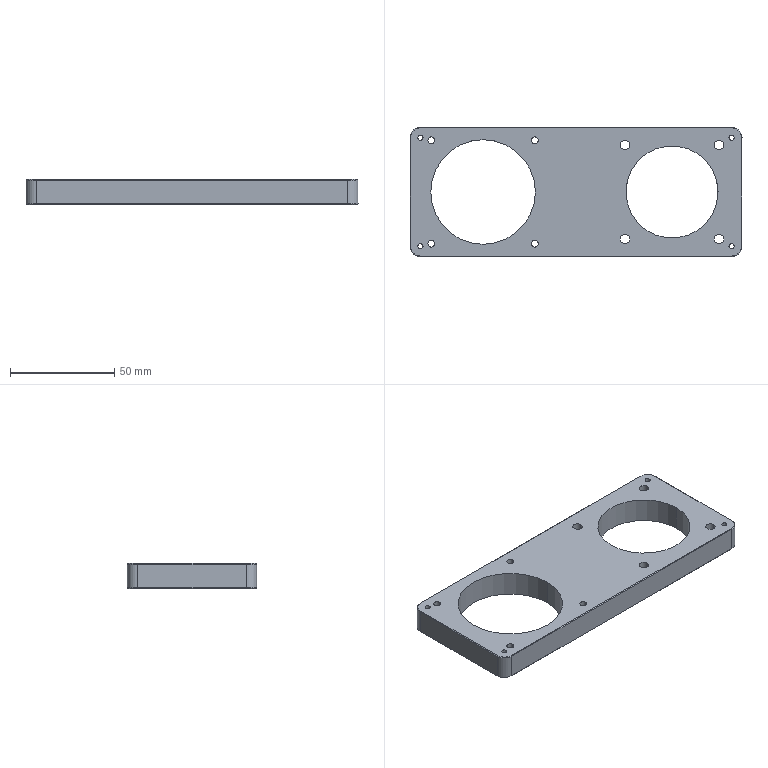Part | SolidWorks | features BaseBody 1 | 1 solid | 66 faces | box 159 x 62 x 12 mm | volume 73972 mm3 | cylinder 40 | plane 18 | cone 8 | commonest cylinder face diameters 2.5 x8 3.3 x8 4.5 x8 8 x8 10 x4 44.1 x2